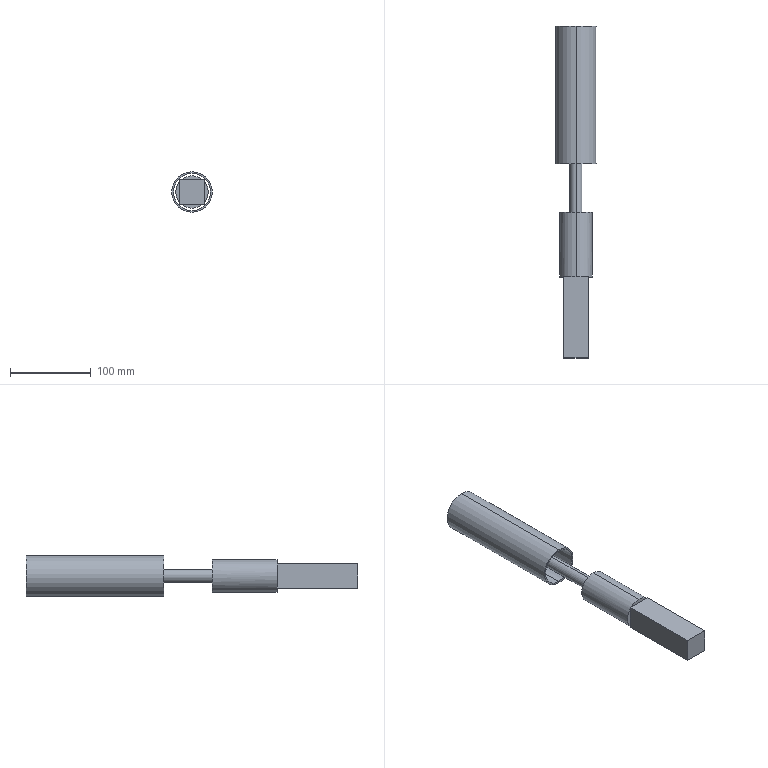Part | SolidWorks | features ICE 3, Extrusion 1 | 2 solids | 25 faces | box 50 x 410 x 50 mm | volume 288046 mm3 | plane 17 | cylinder 8 | commonest cylinder face diameters 16 x2 40 x2 46 x2 50 x2
STEP:
#1=CARTESIAN_POINT('',(0.,60.,-23.));
#2=VERTEX_POINT('',#1);
#3=CARTESIAN_POINT('',(0.,60.,23.));
#4=VERTEX_POINT('',#3);
#5=CARTESIAN_POINT('',(0.,60.,0.));
#6=DIRECTION('',(0.,1.,0.));
#7=DIRECTION('',(0.,0.,1.));
#8=AXIS2_PLACEMENT_3D('',#5,#6,#7);
#9=CIRCLE('',#8,23.);
#10=EDGE_CURVE('',#2,#4,#9,.T.);
#11=ORIENTED_EDGE('',*,*,#10,.F.);
#12=CARTESIAN_POINT('',(0.,230.,-23.));
#13=VERTEX_POINT('',#12);
#14=CARTESIAN_POINT('',(0.,60.,-23.));
#15=DIRECTION('',(0.,1.,0.));
#16=VECTOR('',#15,1000.);
#17=LINE('',#14,#16);
#18=EDGE_CURVE('',#2,#13,#17,.T.);
#19=ORIENTED_EDGE('',*,*,#18,.T.);
#20=CARTESIAN_POINT('',(0.,230.,23.));
#21=VERTEX_POINT('',#20);
#22=CARTESIAN_POINT('',(0.,230.,0.));
#23=DIRECTION('',(0.,1.,0.));
#24=DIRECTION('',(0.,0.,1.));
#25=AXIS2_PLACEMENT_3D('',#22,#23,#24);
#26=CIRCLE('',#25,23.);
#27=EDGE_CURVE('',#13,#21,#26,.T.);
#28=ORIENTED_EDGE('',*,*,#27,.T.);
#29=CARTESIAN_POINT('',(0.,60.,23.));
#30=DIRECTION('',(0.,1.,0.));
#31=VECTOR('',#30,1000.);
#32=LINE('',#29,#31);
#33=EDGE_CURVE('',#4,#21,#32,.T.);
#34=ORIENTED_EDGE('',*,*,#33,.F.);
#35=EDGE_LOOP('',(#11,#19,#28,#34));
#36=FACE_OUTER_BOUND('',#35,.T.);
#37=CARTESIAN_POINT('',(0.,60.,0.));
#38=DIRECTION('',(0.,1.,0.));
#39=DIRECTION('',(0.,0.,1.));
#40=AXIS2_PLACEMENT_3D('',#37,#38,#39);
#41=CYLINDRICAL_SURFACE('',#40,23.);
#42=ADVANCED_FACE('',(#36),#41,.F.);
#43=CARTESIAN_POINT('',(0.,60.,25.));
#44=VERTEX_POINT('',#43);
#45=CARTESIAN_POINT('',(0.,60.,-25.));
#46=VERTEX_POINT('',#45);
#47=CARTESIAN_POINT('',(0.,60.,0.));
#48=DIRECTION('',(0.,1.,0.));
#49=DIRECTION('',(0.,0.,1.));
#50=AXIS2_PLACEMENT_3D('',#47,#48,#49);
#51=CIRCLE('',#50,25.);
#52=EDGE_CURVE('',#44,#46,#51,.T.);
#53=ORIENTED_EDGE('',*,*,#52,.T.);
#54=CARTESIAN_POINT('',(0.,230.,-25.));
#55=VERTEX_POINT('',#54);
#56=CARTESIAN_POINT('',(0.,60.,-25.));
#57=DIRECTION('',(0.,1.,0.));
#58=VECTOR('',#57,1000.);
#59=LINE('',#56,#58);
#60=EDGE_CURVE('',#46,#55,#59,.T.);
#61=ORIENTED_EDGE('',*,*,#60,.T.);
#62=CARTESIAN_POINT('',(0.,230.,25.));
#63=VERTEX_POINT('',#62);
#64=CARTESIAN_POINT('',(0.,230.,0.));
#65=DIRECTION('',(0.,1.,0.));
#66=DIRECTION('',(0.,0.,1.));
#67=AXIS2_PLACEMENT_3D('',#64,#65,#66);
#68=CIRCLE('',#67,25.);
#69=EDGE_CURVE('',#63,#55,#68,.T.);
#70=ORIENTED_EDGE('',*,*,#69,.F.);
#71=CARTESIAN_POINT('',(0.,60.,25.));
#72=DIRECTION('',(0.,1.,0.));
#73=VECTOR('',#72,1000.);
#74=LINE('',#71,#73);
#75=EDGE_CURVE('',#44,#63,#74,.T.);
#76=ORIENTED_EDGE('',*,*,#75,.F.);
#77=EDGE_LOOP('',(#53,#61,#70,#76));
#78=FACE_OUTER_BOUND('',#77,.T.);
#79=CARTESIAN_POINT('',(0.,60.,0.));
#80=DIRECTION('',(0.,1.,0.));
#81=DIRECTION('',(0.,0.,1.));
#82=AXIS2_PLACEMENT_3D('',#79,#80,#81);
#83=CYLINDRICAL_SURFACE('',#82,25.);
#84=ADVANCED_FACE('',(#78),#83,.T.);
#85=ORIENTED_EDGE('',*,*,#60,.F.);
#86=CARTESIAN_POINT('',(0.,60.,0.));
#87=DIRECTION('',(0.,1.,0.));
#88=DIRECTION('',(0.,0.,1.));
#89=AXIS2_PLACEMENT_3D('',#86,#87,#88);
#90=CIRCLE('',#89,25.);
#91=EDGE_CURVE('',#46,#44,#90,.T.);
#92=ORIENTED_EDGE('',*,*,#91,.T.);
#93=ORIENTED_EDGE('',*,*,#75,.T.);
#94=CARTESIAN_POINT('',(0.,230.,0.));
#95=DIRECTION('',(0.,1.,0.));
#96=DIRECTION('',(0.,0.,1.));
#97=AXIS2_PLACEMENT_3D('',#94,#95,#96);
#98=CIRCLE('',#97,25.);
#99=EDGE_CURVE('',#55,#63,#98,.T.);
#100=ORIENTED_EDGE('',*,*,#99,.F.);
#101=EDGE_LOOP('',(#85,#92,#93,#100));
#102=FACE_OUTER_BOUND('',#101,.T.);
#103=CARTESIAN_POINT('',(0.,60.,0.));
#104=DIRECTION('',(0.,1.,0.));
#105=DIRECTION('',(0.,0.,1.));
#106=AXIS2_PLACEMENT_3D('',#103,#104,#105);
#107=CYLINDRICAL_SURFACE('',#106,25.);
#108=ADVANCED_FACE('',(#102),#107,.T.);
#109=CARTESIAN_POINT('',(0.,60.,0.));
#110=DIRECTION('',(0.,1.,0.));
#111=DIRECTION('',(0.,0.,1.));
#112=AXIS2_PLACEMENT_3D('',#109,#110,#111);
#113=CIRCLE('',#112,23.);
#114=EDGE_CURVE('',#4,#2,#113,.T.);
#115=ORIENTED_EDGE('',*,*,#114,.T.);
#116=ORIENTED_EDGE('',*,*,#10,.T.);
#117=EDGE_LOOP('',(#115,#116));
#118=FACE_BOUND('',#117,.T.);
#119=ORIENTED_EDGE('',*,*,#52,.F.);
#120=ORIENTED_EDGE('',*,*,#91,.F.);
#121=EDGE_LOOP('',(#119,#120));
#122=FACE_OUTER_BOUND('',#121,.T.);
#123=CARTESIAN_POINT('',(0.,60.,0.));
#124=DIRECTION('',(0.,1.,0.));
#125=DIRECTION('',(0.,0.,1.));
#126=AXIS2_PLACEMENT_3D('',#123,#124,#125);
#127=PLANE('',#126);
#128=ADVANCED_FACE('',(#118,#122),#127,.F.);
#129=CARTESIAN_POINT('',(0.,230.,0.));
#130=DIRECTION('',(0.,1.,0.));
#131=DIRECTION('',(0.,0.,1.));
#132=AXIS2_PLACEMENT_3D('',#129,#130,#131);
#133=CIRCLE('',#132,23.);
#134=EDGE_CURVE('',#21,#13,#133,.T.);
#135=ORIENTED_EDGE('',*,*,#134,.F.);
#136=ORIENTED_EDGE('',*,*,#27,.F.);
#137=EDGE_LOOP('',(#135,#136));
#138=FACE_BOUND('',#137,.T.);
#139=ORIENTED_EDGE('',*,*,#69,.T.);
#140=ORIENTED_EDGE('',*,*,#99,.T.);
#141=EDGE_LOOP('',(#139,#140));
#142=FACE_OUTER_BOUND('',#141,.T.);
#143=CARTESIAN_POINT('',(0.,230.,0.));
#144=DIRECTION('',(0.,1.,0.));
#145=DIRECTION('',(0.,0.,1.));
#146=AXIS2_PLACEMENT_3D('',#143,#144,#145);
#147=PLANE('',#146);
#148=ADVANCED_FACE('',(#138,#142),#147,.T.);
#149=ORIENTED_EDGE('',*,*,#18,.F.);
#150=ORIENTED_EDGE('',*,*,#114,.F.);
#151=ORIENTED_EDGE('',*,*,#33,.T.);
#152=ORIENTED_EDGE('',*,*,#134,.T.);
#153=EDGE_LOOP('',(#149,#150,#151,#152));
#154=FACE_OUTER_BOUND('',#153,.T.);
#155=CARTESIAN_POINT('',(0.,60.,0.));
#156=DIRECTION('',(0.,1.,0.));
#157=DIRECTION('',(0.,0.,1.));
#158=AXIS2_PLACEMENT_3D('',#155,#156,#157);
#159=CYLINDRICAL_SURFACE('',#158,23.);
#160=ADVANCED_FACE('',(#154),#159,.F.);
#161=CLOSED_SHELL('',(#42,#84,#108,#128,#148,#160));
#162=MANIFOLD_SOLID_BREP('',#161);
#163=CARTESIAN_POINT('',(0.,-80.,-20.));
#164=VERTEX_POINT('',#163);
#165=CARTESIAN_POINT('',(13.229,-80.,-15.));
#166=VERTEX_POINT('',#165);
#167=CARTESIAN_POINT('',(0.,-80.,0.));
#168=DIRECTION('',(0.,-1.,0.));
#169=DIRECTION('',(0.,0.,-1.));
#170=AXIS2_PLACEMENT_3D('',#167,#168,#169);
#171=CIRCLE('',#170,20.);
#172=EDGE_CURVE('',#164,#166,#171,.T.);
#173=ORIENTED_EDGE('',*,*,#172,.F.);
#174=CARTESIAN_POINT('',(0.,0.,-20.));
#175=VERTEX_POINT('',#174);
#176=CARTESIAN_POINT('',(0.,-80.,-20.));
#177=DIRECTION('',(0.,1.,0.));
#178=VECTOR('',#177,1000.);
#179=LINE('',#176,#178);
#180=EDGE_CURVE('',#164,#175,#179,.T.);
#181=ORIENTED_EDGE('',*,*,#180,.T.);
#182=CARTESIAN_POINT('',(0.,0.,20.));
#183=VERTEX_POINT('',#182);
#184=CARTESIAN_POINT('',(0.,0.,0.));
#185=DIRECTION('',(0.,-1.,0.));
#186=DIRECTION('',(0.,0.,-1.));
#187=AXIS2_PLACEMENT_3D('',#184,#185,#186);
#188=CIRCLE('',#187,20.);
#189=EDGE_CURVE('',#175,#183,#188,.T.);
#190=ORIENTED_EDGE('',*,*,#189,.T.);
#191=CARTESIAN_POINT('',(0.,-80.,20.));
#192=VERTEX_POINT('',#191);
#193=CARTESIAN_POINT('',(0.,-80.,20.));
#194=DIRECTION('',(0.,1.,0.));
#195=VECTOR('',#194,1000.);
#196=LINE('',#193,#195);
#197=EDGE_CURVE('',#192,#183,#196,.T.);
#198=ORIENTED_EDGE('',*,*,#197,.F.);
#199=CARTESIAN_POINT('',(13.229,-80.,15.));
#200=VERTEX_POINT('',#199);
#201=CARTESIAN_POINT('',(0.,-80.,0.));
#202=DIRECTION('',(0.,-1.,0.));
#203=DIRECTION('',(0.,0.,-1.));
#204=AXIS2_PLACEMENT_3D('',#201,#202,#203);
#205=CIRCLE('',#204,20.);
#206=EDGE_CURVE('',#200,#192,#205,.T.);
#207=ORIENTED_EDGE('',*,*,#206,.F.);
#208=CARTESIAN_POINT('',(15.,-80.,13.229));
#209=VERTEX_POINT('',#208);
#210=CARTESIAN_POINT('',(0.,-80.,0.));
#211=DIRECTION('',(0.,-1.,0.));
#212=DIRECTION('',(0.,0.,-1.));
#213=AXIS2_PLACEMENT_3D('',#210,#211,#212);
#214=CIRCLE('',#213,20.);
#215=EDGE_CURVE('',#209,#200,#214,.T.);
#216=ORIENTED_EDGE('',*,*,#215,.F.);
#217=CARTESIAN_POINT('',(15.,-80.,-13.229));
#218=VERTEX_POINT('',#217);
#219=CARTESIAN_POINT('',(0.,-80.,0.));
#220=DIRECTION('',(0.,-1.,0.));
#221=DIRECTION('',(0.,0.,-1.));
#222=AXIS2_PLACEMENT_3D('',#219,#220,#221);
#223=CIRCLE('',#222,20.);
#224=EDGE_CURVE('',#218,#209,#223,.T.);
#225=ORIENTED_EDGE('',*,*,#224,.F.);
#226=CARTESIAN_POINT('',(0.,-80.,0.));
#227=DIRECTION('',(0.,-1.,0.));
#228=DIRECTION('',(0.,0.,-1.));
#229=AXIS2_PLACEMENT_3D('',#226,#227,#228);
#230=CIRCLE('',#229,20.);
#231=EDGE_CURVE('',#166,#218,#230,.T.);
#232=ORIENTED_EDGE('',*,*,#231,.F.);
#233=EDGE_LOOP('',(#173,#181,#190,#198,#207,#216,#225,#232));
#234=FACE_OUTER_BOUND('',#233,.T.);
#235=CARTESIAN_POINT('',(0.,-80.,0.));
#236=DIRECTION('',(0.,1.,0.));
#237=DIRECTION('',(0.,0.,1.));
#238=AXIS2_PLACEMENT_3D('',#235,#236,#237);
#239=CYLINDRICAL_SURFACE('',#238,20.);
#240=ADVANCED_FACE('',(#234),#239,.T.);
#241=CARTESIAN_POINT('',(0.,230.,8.));
#242=VERTEX_POINT('',#241);
#243=CARTESIAN_POINT('',(0.,230.,-8.));
#244=VERTEX_POINT('',#243);
#245=CARTESIAN_POINT('',(0.,230.,0.));
#246=DIRECTION('',(0.,1.,0.));
#247=DIRECTION('',(0.,0.,1.));
#248=AXIS2_PLACEMENT_3D('',#245,#246,#247);
#249=CIRCLE('',#248,8.);
#250=EDGE_CURVE('',#242,#244,#249,.T.);
#251=ORIENTED_EDGE('',*,*,#250,.F.);
#252=CARTESIAN_POINT('',(0.,0.,8.));
#253=VERTEX_POINT('',#252);
#254=CARTESIAN_POINT('',(0.,230.,8.));
#255=DIRECTION('',(0.,-1.,0.));
#256=VECTOR('',#255,1000.);
#257=LINE('',#254,#256);
#258=EDGE_CURVE('',#242,#253,#257,.T.);
#259=ORIENTED_EDGE('',*,*,#258,.T.);
#260=CARTESIAN_POINT('',(0.,0.,-8.));
#261=VERTEX_POINT('',#260);
#262=CARTESIAN_POINT('',(0.,0.,0.));
#263=DIRECTION('',(0.,1.,0.));
#264=DIRECTION('',(0.,0.,1.));
#265=AXIS2_PLACEMENT_3D('',#262,#263,#264);
#266=CIRCLE('',#265,8.);
#267=EDGE_CURVE('',#253,#261,#266,.T.);
#268=ORIENTED_EDGE('',*,*,#267,.T.);
#269=CARTESIAN_POINT('',(0.,230.,-8.));
#270=DIRECTION('',(0.,-1.,0.));
#271=VECTOR('',#270,1000.);
#272=LINE('',#269,#271);
#273=EDGE_CURVE('',#244,#261,#272,.T.);
#274=ORIENTED_EDGE('',*,*,#273,.F.);
#275=EDGE_LOOP('',(#251,#259,#268,#274));
#276=FACE_OUTER_BOUND('',#275,.T.);
#277=CARTESIAN_POINT('',(0.,230.,0.));
#278=DIRECTION('',(0.,-1.,0.));
#279=DIRECTION('',(0.,0.,-1.));
#280=AXIS2_PLACEMENT_3D('',#277,#278,#279);
#281=CYLINDRICAL_SURFACE('',#280,8.);
#282=ADVANCED_FACE('',(#276),#281,.T.);
#283=CARTESIAN_POINT('',(15.,-80.,15.));
#284=DIRECTION('',(0.,0.,1.));
#285=VECTOR('',#284,1000.);
#286=LINE('',#283,#285);
#287=EDGE_CURVE('',#218,#209,#286,.T.);
#288=ORIENTED_EDGE('',*,*,#287,.F.);
#289=ORIENTED_EDGE('',*,*,#224,.T.);
#290=EDGE_LOOP('',(#288,#289));
#291=FACE_OUTER_BOUND('',#290,.T.);
#292=CARTESIAN_POINT('',(0.,-80.,0.));
#293=DIRECTION('',(0.,-1.,0.));
#294=DIRECTION('',(0.,0.,-1.));
#295=AXIS2_PLACEMENT_3D('',#292,#293,#294);
#296=PLANE('',#295);
#297=ADVANCED_FACE('',(#291),#296,.T.);
#298=CARTESIAN_POINT('',(-13.229,-80.,-15.));
#299=VERTEX_POINT('',#298);
#300=CARTESIAN_POINT('',(-15.,-80.,-15.));
#301=DIRECTION('',(1.,0.,0.));
#302=VECTOR('',#301,1000.);
#303=LINE('',#300,#302);
#304=EDGE_CURVE('',#299,#166,#303,.T.);
#305=ORIENTED_EDGE('',*,*,#304,.F.);
#306=CARTESIAN_POINT('',(0.,-80.,0.));
#307=DIRECTION('',(0.,-1.,0.));
#308=DIRECTION('',(0.,0.,-1.));
#309=AXIS2_PLACEMENT_3D('',#306,#307,#308);
#310=CIRCLE('',#309,20.);
#311=EDGE_CURVE('',#299,#164,#310,.T.);
#312=ORIENTED_EDGE('',*,*,#311,.T.);
#313=ORIENTED_EDGE('',*,*,#172,.T.);
#314=EDGE_LOOP('',(#305,#312,#313));
#315=FACE_OUTER_BOUND('',#314,.T.);
#316=CARTESIAN_POINT('',(0.,-80.,0.));
#317=DIRECTION('',(0.,-1.,0.));
#318=DIRECTION('',(0.,0.,-1.));
#319=AXIS2_PLACEMENT_3D('',#316,#317,#318);
#320=PLANE('',#319);
#321=ADVANCED_FACE('',(#315),#320,.T.);
#322=CARTESIAN_POINT('',(-15.,-80.,13.229));
#323=VERTEX_POINT('',#322);
#324=CARTESIAN_POINT('',(-15.,-80.,-13.229));
#325=VERTEX_POINT('',#324);
#326=CARTESIAN_POINT('',(-15.,-80.,15.));
#327=DIRECTION('',(0.,0.,-1.));
#328=VECTOR('',#327,1000.);
#329=LINE('',#326,#328);
#330=EDGE_CURVE('',#323,#325,#329,.T.);
#331=ORIENTED_EDGE('',*,*,#330,.F.);
#332=CARTESIAN_POINT('',(0.,-80.,0.));
#333=DIRECTION('',(0.,-1.,0.));
#334=DIRECTION('',(0.,0.,-1.));
#335=AXIS2_PLACEMENT_3D('',#332,#333,#334);
#336=CIRCLE('',#335,20.);
#337=EDGE_CURVE('',#323,#325,#336,.T.);
#338=ORIENTED_EDGE('',*,*,#337,.T.);
#339=EDGE_LOOP('',(#331,#338));
#340=FACE_OUTER_BOUND('',#339,.T.);
#341=CARTESIAN_POINT('',(0.,-80.,0.));
#342=DIRECTION('',(0.,-1.,0.));
#343=DIRECTION('',(0.,0.,-1.));
#344=AXIS2_PLACEMENT_3D('',#341,#342,#343);
#345=PLANE('',#344);
#346=ADVANCED_FACE('',(#340),#345,.T.);
#347=ORIENTED_EDGE('',*,*,#258,.F.);
#348=CARTESIAN_POINT('',(0.,230.,0.));
#349=DIRECTION('',(0.,1.,0.));
#350=DIRECTION('',(0.,0.,1.));
#351=AXIS2_PLACEMENT_3D('',#348,#349,#350);
#352=CIRCLE('',#351,8.);
#353=EDGE_CURVE('',#244,#242,#352,.T.);
#354=ORIENTED_EDGE('',*,*,#353,.F.);
#355=ORIENTED_EDGE('',*,*,#273,.T.);
#356=CARTESIAN_POINT('',(0.,0.,0.));
#357=DIRECTION('',(0.,1.,0.));
#358=DIRECTION('',(0.,0.,1.));
#359=AXIS2_PLACEMENT_3D('',#356,#357,#358);
#360=CIRCLE('',#359,8.);
#361=EDGE_CURVE('',#261,#253,#360,.T.);
#362=ORIENTED_EDGE('',*,*,#361,.T.);
#363=EDGE_LOOP('',(#347,#354,#355,#362));
#364=FACE_OUTER_BOUND('',#363,.T.);
#365=CARTESIAN_POINT('',(0.,230.,0.));
#366=DIRECTION('',(0.,-1.,0.));
#367=DIRECTION('',(0.,0.,-1.));
#368=AXIS2_PLACEMENT_3D('',#365,#366,#367);
#369=CYLINDRICAL_SURFACE('',#368,8.);
#370=ADVANCED_FACE('',(#364),#369,.T.);
#371=ORIENTED_EDGE('',*,*,#353,.T.);
#372=ORIENTED_EDGE('',*,*,#250,.T.);
#373=EDGE_LOOP('',(#371,#372));
#374=FACE_OUTER_BOUND('',#373,.T.);
#375=CARTESIAN_POINT('',(0.,230.,0.));
#376=DIRECTION('',(0.,1.,0.));
#377=DIRECTION('',(0.,0.,1.));
#378=AXIS2_PLACEMENT_3D('',#375,#376,#377);
#379=PLANE('',#378);
#380=ADVANCED_FACE('',(#374),#379,.T.);
#381=ORIENTED_EDGE('',*,*,#180,.F.);
#382=ORIENTED_EDGE('',*,*,#311,.F.);
#383=CARTESIAN_POINT('',(0.,-80.,0.));
#384=DIRECTION('',(0.,-1.,0.));
#385=DIRECTION('',(0.,0.,-1.));
#386=AXIS2_PLACEMENT_3D('',#383,#384,#385);
#387=CIRCLE('',#386,20.);
#388=EDGE_CURVE('',#325,#299,#387,.T.);
#389=ORIENTED_EDGE('',*,*,#388,.F.);
#390=ORIENTED_EDGE('',*,*,#337,.F.);
#391=CARTESIAN_POINT('',(-13.229,-80.,15.));
#392=VERTEX_POINT('',#391);
#393=CARTESIAN_POINT('',(0.,-80.,0.));
#394=DIRECTION('',(0.,-1.,0.));
#395=DIRECTION('',(0.,0.,-1.));
#396=AXIS2_PLACEMENT_3D('',#393,#394,#395);
#397=CIRCLE('',#396,20.);
#398=EDGE_CURVE('',#392,#323,#397,.T.);
#399=ORIENTED_EDGE('',*,*,#398,.F.);
#400=CARTESIAN_POINT('',(0.,-80.,0.));
#401=DIRECTION('',(0.,-1.,0.));
#402=DIRECTION('',(0.,0.,-1.));
#403=AXIS2_PLACEMENT_3D('',#400,#401,#402);
#404=CIRCLE('',#403,20.);
#405=EDGE_CURVE('',#192,#392,#404,.T.);
#406=ORIENTED_EDGE('',*,*,#405,.F.);
#407=ORIENTED_EDGE('',*,*,#197,.T.);
#408=CARTESIAN_POINT('',(0.,0.,0.));
#409=DIRECTION('',(0.,-1.,0.));
#410=DIRECTION('',(0.,0.,-1.));
#411=AXIS2_PLACEMENT_3D('',#408,#409,#410);
#412=CIRCLE('',#411,20.);
#413=EDGE_CURVE('',#183,#175,#412,.T.);
#414=ORIENTED_EDGE('',*,*,#413,.T.);
#415=EDGE_LOOP('',(#381,#382,#389,#390,#399,#406,#407,#414));
#416=FACE_OUTER_BOUND('',#415,.T.);
#417=CARTESIAN_POINT('',(0.,-80.,0.));
#418=DIRECTION('',(0.,1.,0.));
#419=DIRECTION('',(0.,0.,1.));
#420=AXIS2_PLACEMENT_3D('',#417,#418,#419);
#421=CYLINDRICAL_SURFACE('',#420,20.);
#422=ADVANCED_FACE('',(#416),#421,.T.);
#423=CARTESIAN_POINT('',(-15.,-80.,15.));
#424=DIRECTION('',(-1.,0.,0.));
#425=VECTOR('',#424,1000.);
#426=LINE('',#423,#425);
#427=EDGE_CURVE('',#200,#392,#426,.T.);
#428=ORIENTED_EDGE('',*,*,#427,.F.);
#429=ORIENTED_EDGE('',*,*,#206,.T.);
#430=ORIENTED_EDGE('',*,*,#405,.T.);
#431=EDGE_LOOP('',(#428,#429,#430));
#432=FACE_OUTER_BOUND('',#431,.T.);
#433=CARTESIAN_POINT('',(0.,-80.,0.));
#434=DIRECTION('',(0.,-1.,0.));
#435=DIRECTION('',(0.,0.,-1.));
#436=AXIS2_PLACEMENT_3D('',#433,#434,#435);
#437=PLANE('',#436);
#438=ADVANCED_FACE('',(#432),#437,.T.);
#439=ORIENTED_EDGE('',*,*,#361,.F.);
#440=ORIENTED_EDGE('',*,*,#267,.F.);
#441=EDGE_LOOP('',(#439,#440));
#442=FACE_BOUND('',#441,.T.);
#443=ORIENTED_EDGE('',*,*,#413,.F.);
#444=ORIENTED_EDGE('',*,*,#189,.F.);
#445=EDGE_LOOP('',(#443,#444));
#446=FACE_OUTER_BOUND('',#445,.T.);
#447=CARTESIAN_POINT('',(0.,0.,0.));
#448=DIRECTION('',(0.,-1.,0.));
#449=DIRECTION('',(0.,0.,-1.));
#450=AXIS2_PLACEMENT_3D('',#447,#448,#449);
#451=PLANE('',#450);
#452=ADVANCED_FACE('',(#442,#446),#451,.F.);
#453=CARTESIAN_POINT('',(15.,-80.,-15.));
#454=VERTEX_POINT('',#453);
#455=CARTESIAN_POINT('',(-15.,-80.,-15.));
#456=DIRECTION('',(1.,0.,0.));
#457=VECTOR('',#456,1000.);
#458=LINE('',#455,#457);
#459=EDGE_CURVE('',#166,#454,#458,.T.);
#460=ORIENTED_EDGE('',*,*,#459,.F.);
#461=ORIENTED_EDGE('',*,*,#231,.T.);
#462=CARTESIAN_POINT('',(15.,-80.,15.));
#463=DIRECTION('',(0.,0.,1.));
#464=VECTOR('',#463,1000.);
#465=LINE('',#462,#464);
#466=EDGE_CURVE('',#454,#218,#465,.T.);
#467=ORIENTED_EDGE('',*,*,#466,.F.);
#468=EDGE_LOOP('',(#460,#461,#467));
#469=FACE_OUTER_BOUND('',#468,.T.);
#470=CARTESIAN_POINT('',(0.,-80.,0.));
#471=DIRECTION('',(0.,-1.,0.));
#472=DIRECTION('',(0.,0.,-1.));
#473=AXIS2_PLACEMENT_3D('',#470,#471,#472);
#474=PLANE('',#473);
#475=ADVANCED_FACE('',(#469),#474,.F.);
#476=CARTESIAN_POINT('',(15.,-80.,15.));
#477=VERTEX_POINT('',#476);
#478=CARTESIAN_POINT('',(15.,-80.,15.));
#479=DIRECTION('',(0.,0.,1.));
#480=VECTOR('',#479,1000.);
#481=LINE('',#478,#480);
#482=EDGE_CURVE('',#209,#477,#481,.T.);
#483=ORIENTED_EDGE('',*,*,#482,.F.);
#484=ORIENTED_EDGE('',*,*,#215,.T.);
#485=CARTESIAN_POINT('',(-15.,-80.,15.));
#486=DIRECTION('',(-1.,0.,0.));
#487=VECTOR('',#486,1000.);
#488=LINE('',#485,#487);
#489=EDGE_CURVE('',#477,#200,#488,.T.);
#490=ORIENTED_EDGE('',*,*,#489,.F.);
#491=EDGE_LOOP('',(#483,#484,#490));
#492=FACE_OUTER_BOUND('',#491,.T.);
#493=CARTESIAN_POINT('',(0.,-80.,0.));
#494=DIRECTION('',(0.,-1.,0.));
#495=DIRECTION('',(0.,0.,-1.));
#496=AXIS2_PLACEMENT_3D('',#493,#494,#495);
#497=PLANE('',#496);
#498=ADVANCED_FACE('',(#492),#497,.F.);
#499=CARTESIAN_POINT('',(-15.,-80.,15.));
#500=VERTEX_POINT('',#499);
#501=CARTESIAN_POINT('',(-15.,-80.,15.));
#502=DIRECTION('',(-1.,0.,0.));
#503=VECTOR('',#502,1000.);
#504=LINE('',#501,#503);
#505=EDGE_CURVE('',#392,#500,#504,.T.);
#506=ORIENTED_EDGE('',*,*,#505,.F.);
#507=ORIENTED_EDGE('',*,*,#398,.T.);
#508=CARTESIAN_POINT('',(-15.,-80.,15.));
#509=DIRECTION('',(0.,0.,-1.));
#510=VECTOR('',#509,1000.);
#511=LINE('',#508,#510);
#512=EDGE_CURVE('',#500,#323,#511,.T.);
#513=ORIENTED_EDGE('',*,*,#512,.F.);
#514=EDGE_LOOP('',(#506,#507,#513));
#515=FACE_OUTER_BOUND('',#514,.T.);
#516=CARTESIAN_POINT('',(0.,-80.,0.));
#517=DIRECTION('',(0.,-1.,0.));
#518=DIRECTION('',(0.,0.,-1.));
#519=AXIS2_PLACEMENT_3D('',#516,#517,#518);
#520=PLANE('',#519);
#521=ADVANCED_FACE('',(#515),#520,.F.);
#522=CARTESIAN_POINT('',(-15.,-80.,-15.));
#523=VERTEX_POINT('',#522);
#524=CARTESIAN_POINT('',(-15.,-80.,15.));
#525=DIRECTION('',(0.,0.,-1.));
#526=VECTOR('',#525,1000.);
#527=LINE('',#524,#526);
#528=EDGE_CURVE('',#325,#523,#527,.T.);
#529=ORIENTED_EDGE('',*,*,#528,.F.);
#530=ORIENTED_EDGE('',*,*,#388,.T.);
#531=CARTESIAN_POINT('',(-15.,-80.,-15.));
#532=DIRECTION('',(1.,0.,0.));
#533=VECTOR('',#532,1000.);
#534=LINE('',#531,#533);
#535=EDGE_CURVE('',#523,#299,#534,.T.);
#536=ORIENTED_EDGE('',*,*,#535,.F.);
#537=EDGE_LOOP('',(#529,#530,#536));
#538=FACE_OUTER_BOUND('',#537,.T.);
#539=CARTESIAN_POINT('',(0.,-80.,0.));
#540=DIRECTION('',(0.,-1.,0.));
#541=DIRECTION('',(0.,0.,-1.));
#542=AXIS2_PLACEMENT_3D('',#539,#540,#541);
#543=PLANE('',#542);
#544=ADVANCED_FACE('',(#538),#543,.F.);
#545=ORIENTED_EDGE('',*,*,#466,.T.);
#546=ORIENTED_EDGE('',*,*,#287,.T.);
#547=ORIENTED_EDGE('',*,*,#482,.T.);
#548=CARTESIAN_POINT('',(15.,-180.,15.));
#549=VERTEX_POINT('',#548);
#550=CARTESIAN_POINT('',(15.,-180.,15.));
#551=DIRECTION('',(0.,1.,0.));
#552=VECTOR('',#551,1000.);
#553=LINE('',#550,#552);
#554=EDGE_CURVE('',#549,#477,#553,.T.);
#555=ORIENTED_EDGE('',*,*,#554,.F.);
#556=CARTESIAN_POINT('',(15.,-180.,-15.));
#557=VERTEX_POINT('',#556);
#558=CARTESIAN_POINT('',(15.,-180.,15.));
#559=DIRECTION('',(0.,0.,1.));
#560=VECTOR('',#559,1000.);
#561=LINE('',#558,#560);
#562=EDGE_CURVE('',#557,#549,#561,.T.);
#563=ORIENTED_EDGE('',*,*,#562,.F.);
#564=CARTESIAN_POINT('',(15.,-180.,-15.));
#565=DIRECTION('',(0.,1.,0.));
#566=VECTOR('',#565,1000.);
#567=LINE('',#564,#566);
#568=EDGE_CURVE('',#557,#454,#567,.T.);
#569=ORIENTED_EDGE('',*,*,#568,.T.);
#570=EDGE_LOOP('',(#545,#546,#547,#555,#563,#569));
#571=FACE_OUTER_BOUND('',#570,.T.);
#572=CARTESIAN_POINT('',(15.,-180.,15.));
#573=DIRECTION('',(-1.,0.,0.));
#574=DIRECTION('',(0.,0.,1.));
#575=AXIS2_PLACEMENT_3D('',#572,#573,#574);
#576=PLANE('',#575);
#577=ADVANCED_FACE('',(#571),#576,.F.);
#578=ORIENTED_EDGE('',*,*,#489,.T.);
#579=ORIENTED_EDGE('',*,*,#427,.T.);
#580=ORIENTED_EDGE('',*,*,#505,.T.);
#581=CARTESIAN_POINT('',(-15.,-180.,15.));
#582=VERTEX_POINT('',#581);
#583=CARTESIAN_POINT('',(-15.,-180.,15.));
#584=DIRECTION('',(0.,1.,0.));
#585=VECTOR('',#584,1000.);
#586=LINE('',#583,#585);
#587=EDGE_CURVE('',#582,#500,#586,.T.);
#588=ORIENTED_EDGE('',*,*,#587,.F.);
#589=CARTESIAN_POINT('',(-15.,-180.,15.));
#590=DIRECTION('',(-1.,0.,0.));
#591=VECTOR('',#590,1000.);
#592=LINE('',#589,#591);
#593=EDGE_CURVE('',#549,#582,#592,.T.);
#594=ORIENTED_EDGE('',*,*,#593,.F.);
#595=ORIENTED_EDGE('',*,*,#554,.T.);
#596=EDGE_LOOP('',(#578,#579,#580,#588,#594,#595));
#597=FACE_OUTER_BOUND('',#596,.T.);
#598=CARTESIAN_POINT('',(-15.,-180.,15.));
#599=DIRECTION('',(0.,0.,-1.));
#600=DIRECTION('',(-1.,0.,0.));
#601=AXIS2_PLACEMENT_3D('',#598,#599,#600);
#602=PLANE('',#601);
#603=ADVANCED_FACE('',(#597),#602,.F.);
#604=ORIENTED_EDGE('',*,*,#512,.T.);
#605=ORIENTED_EDGE('',*,*,#330,.T.);
#606=ORIENTED_EDGE('',*,*,#528,.T.);
#607=CARTESIAN_POINT('',(-15.,-180.,-15.));
#608=VERTEX_POINT('',#607);
#609=CARTESIAN_POINT('',(-15.,-180.,-15.));
#610=DIRECTION('',(0.,1.,0.));
#611=VECTOR('',#610,1000.);
#612=LINE('',#609,#611);
#613=EDGE_CURVE('',#608,#523,#612,.T.);
#614=ORIENTED_EDGE('',*,*,#613,.F.);
#615=CARTESIAN_POINT('',(-15.,-180.,15.));
#616=DIRECTION('',(0.,0.,-1.));
#617=VECTOR('',#616,1000.);
#618=LINE('',#615,#617);
#619=EDGE_CURVE('',#582,#608,#618,.T.);
#620=ORIENTED_EDGE('',*,*,#619,.F.);
#621=ORIENTED_EDGE('',*,*,#587,.T.);
#622=EDGE_LOOP('',(#604,#605,#606,#614,#620,#621));
#623=FACE_OUTER_BOUND('',#622,.T.);
#624=CARTESIAN_POINT('',(-15.,-180.,15.));
#625=DIRECTION('',(1.,0.,0.));
#626=DIRECTION('',(0.,0.,-1.));
#627=AXIS2_PLACEMENT_3D('',#624,#625,#626);
#628=PLANE('',#627);
#629=ADVANCED_FACE('',(#623),#628,.F.);
#630=ORIENTED_EDGE('',*,*,#535,.T.);
#631=ORIENTED_EDGE('',*,*,#304,.T.);
#632=ORIENTED_EDGE('',*,*,#459,.T.);
#633=ORIENTED_EDGE('',*,*,#568,.F.);
#634=CARTESIAN_POINT('',(-15.,-180.,-15.));
#635=DIRECTION('',(1.,0.,0.));
#636=VECTOR('',#635,1000.);
#637=LINE('',#634,#636);
#638=EDGE_CURVE('',#608,#557,#637,.T.);
#639=ORIENTED_EDGE('',*,*,#638,.F.);
#640=ORIENTED_EDGE('',*,*,#613,.T.);
#641=EDGE_LOOP('',(#630,#631,#632,#633,#639,#640));
#642=FACE_OUTER_BOUND('',#641,.T.);
#643=CARTESIAN_POINT('',(-15.,-180.,-15.));
#644=DIRECTION('',(0.,0.,1.));
#645=DIRECTION('',(1.,0.,0.));
#646=AXIS2_PLACEMENT_3D('',#643,#644,#645);
#647=PLANE('',#646);
#648=ADVANCED_FACE('',(#642),#647,.F.);
#649=ORIENTED_EDGE('',*,*,#562,.T.);
#650=ORIENTED_EDGE('',*,*,#593,.T.);
#651=ORIENTED_EDGE('',*,*,#619,.T.);
#652=ORIENTED_EDGE('',*,*,#638,.T.);
#653=EDGE_LOOP('',(#649,#650,#651,#652));
#654=FACE_OUTER_BOUND('',#653,.T.);
#655=CARTESIAN_POINT('',(0.,-180.,0.));
#656=DIRECTION('',(0.,-1.,0.));
#657=DIRECTION('',(0.,0.,-1.));
#658=AXIS2_PLACEMENT_3D('',#655,#656,#657);
#659=PLANE('',#658);
#660=ADVANCED_FACE('',(#654),#659,.T.);
#661=CLOSED_SHELL('',(#240,#282,#297,#321,#346,#370,#380,#422,#438,#452,#475,#498,#521,#544,#577,#603,#629,#648,#660));
#662=MANIFOLD_SOLID_BREP('',#661);
#663=CARTESIAN_POINT('',(0.,0.,0.));
#664=DIRECTION('',(0.,0.,1.));
#665=DIRECTION('',(1.,0.,0.));
#666=AXIS2_PLACEMENT_3D('',#663,#664,#665);
#667=(LENGTH_UNIT()NAMED_UNIT(*)SI_UNIT(.MILLI.,.METRE.));
#668=UNCERTAINTY_MEASURE_WITH_UNIT(LENGTH_MEASURE(0.00001),#667,'','');
#669=(NAMED_UNIT(*)PLANE_ANGLE_UNIT()SI_UNIT($,.RADIAN.));
#670=(NAMED_UNIT(*)SI_UNIT($,.STERADIAN.)SOLID_ANGLE_UNIT());
#671=(GEOMETRIC_REPRESENTATION_CONTEXT(3)GLOBAL_UNCERTAINTY_ASSIGNED_CONTEXT((#668))GLOBAL_UNIT_ASSIGNED_CONTEXT((#667,#669,#670))REPRESENTATION_CONTEXT('',''));
#672=ADVANCED_BREP_SHAPE_REPRESENTATION('',(#162,#662,#666),#671);